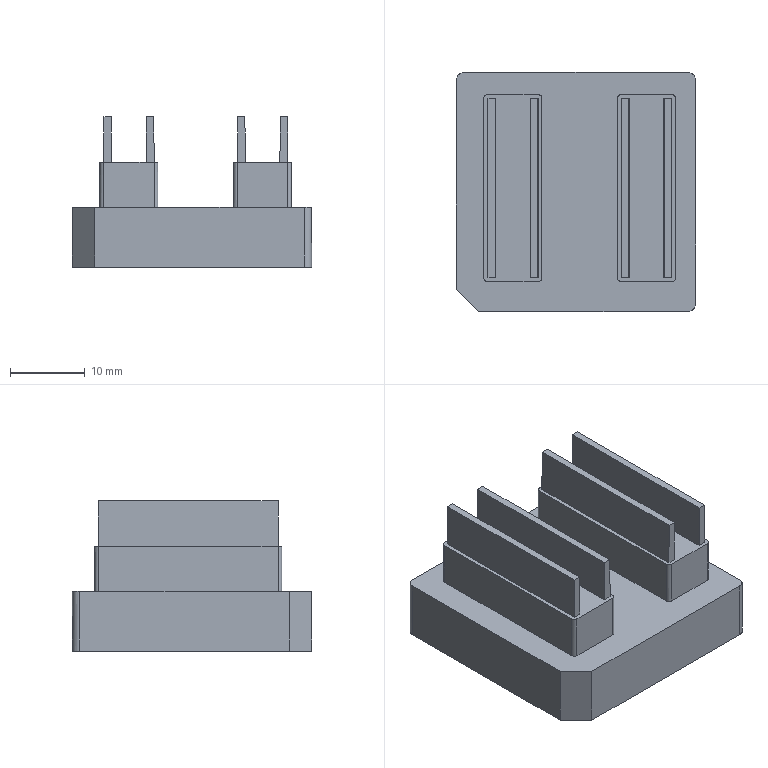NC program | PowerMill | posted with a generic post | part box 32 x 32 x 20.109 mm
Lines 5927 to 6909 of 124326:
N6024 M6
N6025 S18000 M03
N6026 G00 G90 X0.0 Y0.0
N6027 G43 Z9.7992 H10
N6028
N6029 G05 P10000 R4
N6030 X-8.0366 Y14.4474
N6031 Z0.8417
N6032 G01 Z-0.3583 F3000.0
N6033 X-8.0407 Y14.4286 F5000.0
N6034 G03 X-7.9079 Y14.2227 I0.1694 J-0.0366
N6035 G01 X-6.5639 Y13.9322
N6036 X-6.332 Y13.9917
N6037 X-5.0656 Y14.0127
N6038 X-4.6435 Y13.9367
N6039 X-4.2213 Y13.7119
N6040 X-3.9916 Y13.5083
N6041 X-3.7992 Y13.2347
N6042 X-3.7268 Y13.0861
N6043 X-3.6258 Y12.664
N6044 X-3.6132 Y12.2419
N6045 Y-11.3976
N6046 X-3.6515 Y-11.8197
N6047 X-3.7992 Y-12.2357
N6048 X-4.155 Y-12.664
N6049 X-4.6435 Y-12.9367
N6050 X-5.0656 Y-13.0127
N6051 X-6.332 Y-12.992
N6052 X-6.7541 Y-12.8517
N6053 X-7.0361 Y-12.664
N6054 X-7.1763 Y-12.536
N6055 X-7.3878 Y-12.2419
N6056 X-7.545 Y-11.8197
N6057 X-7.578 Y-11.3976
N6058 Y12.2419
N6059 X-7.5711 Y12.664
N6060 X-7.4587 Y13.0861
N6061 X-7.1989 Y13.5083
N6062 X-6.7541 Y13.8445
N6063 X-6.5711 Y13.9304
N6064 X-6.5639 Y13.9322
N6065 X-9.1258 Y14.4424
N6066 X-9.1676 Y14.2545
N6067 X-9.4274 Y13.0861
N6068 X-9.322 Y12.664
N6069 X-9.3158 Y12.2419
N6070 Y-11.3976
N6071 X-9.3507 Y-11.8197
N6072 X-9.5077 Y-12.2419
N6073 X-9.7091 Y-12.5237
N6074 X-9.8512 Y-12.664
N6075 X-10.1312 Y-12.8478
N6076 X-10.5533 Y-12.9903
N6077 X-10.9755 Y-13.0134
N6078 X-11.8197 Y-13.0124
N6079 X-12.2419 Y-12.9398
N6080 X-12.664 Y-12.7219
N6081 X-13.0861 Y-12.2457
N6082 X-13.2442 Y-11.8197
N6083 X-13.2724 Y-11.3976
N6084 X-13.2704 Y12.664
N6085 X-13.1589 Y13.0861
N6086 X-13.0861 Y13.2475
N6087 X-12.9007 Y13.5083
N6088 X-12.664 Y13.7232
N6089 X-12.2636 Y13.9304
N6090 X-11.8197 Y14.0127
N6091 X-10.9755 Y14.0134
N6092 X-10.5533 Y13.9902
N6093 X-10.3233 Y13.9304
N6094 X-10.1312 Y13.8488
N6095 X-9.7091 Y13.525
N6096 X-9.4274 Y13.0861
N6097 X-8.0426 Y14.447 Z-0.5056
N6098 X-8.0466 Y14.4282
N6099 G03 X-7.9139 Y14.2222 I0.1693 J-0.0367
N6100 G01 X-6.5688 Y13.9313
N6101 X-6.332 Y13.992
N6102 X-5.0656 Y14.0127
N6103 X-4.6435 Y13.9379
N6104 X-4.2213 Y13.7157
N6105 X-3.99 Y13.5083
N6106 X-3.7992 Y13.2376
N6107 X-3.7255 Y13.0861
N6108 X-3.6236 Y12.664
N6109 X-3.6119 Y12.2419
N6110 Y-11.3976
N6111 X-3.6467 Y-11.8197
N6112 X-3.7992 Y-12.2386
N6113 X-4.1495 Y-12.664
N6114 X-4.6435 Y-12.9375
N6115 X-5.0656 Y-13.0127
N6116 X-6.332 Y-12.9922
N6117 X-6.7541 Y-12.8531
N6118 X-7.0383 Y-12.664
N6119 X-7.1763 Y-12.5374
N6120 X-7.3908 Y-12.2419
N6121 X-7.5485 Y-11.8197
N6122 X-7.5795 Y-11.3976
N6123 Y12.2419
N6124 X-7.5724 Y12.664
N6125 X-7.4617 Y13.0861
N6126 X-7.2013 Y13.5083
N6127 X-6.7541 Y13.8486
N6128 X-6.5724 Y13.9304
N6129 X-6.5688 Y13.9313
N6130 X-9.1247 Y14.4437
N6131 X-9.1662 Y14.2557
N6132 X-9.4247 Y13.0861
N6133 X-9.3187 Y12.664
N6134 X-9.3111 Y12.2419
N6135 Y-11.3976
N6136 X-9.3471 Y-11.8197
N6137 X-9.5043 Y-12.2419
N6138 X-9.7091 Y-12.5265
N6139 X-9.8496 Y-12.664
N6140 X-10.1312 Y-12.8505
N6141 X-10.5533 Y-12.9912
N6142 X-10.9755 Y-13.0134
N6143 X-11.8197 Y-13.0128
N6144 X-12.2419 Y-12.9403
N6145 X-12.664 Y-12.7233
N6146 X-12.7378 Y-12.664
N6147 X-13.0861 Y-12.2492
N6148 X-13.2466 Y-11.8197
N6149 X-13.2748 Y-11.3976
N6150 X-13.2717 Y12.664
N6151 X-13.1613 Y13.0861
N6152 X-13.0861 Y13.2497
N6153 X-12.9019 Y13.5083
N6154 X-12.664 Y13.7243
N6155 X-12.2673 Y13.9304
N6156 X-11.8197 Y14.0128
N6157 X-10.9755 Y14.0134
N6158 X-10.5533 Y13.9908
N6159 X-10.3188 Y13.9304
N6160 X-10.1312 Y13.8502
N6161 X-9.7091 Y13.5273
N6162 X-9.4247 Y13.0861
N6163 X-8.0446 Y14.4474 Z-0.6529
N6164 X-8.0486 Y14.4286
N6165 G03 X-7.916 Y14.2226 I0.1693 J-0.0367
N6166 G01 X-6.57 Y13.9313
N6167 X-6.332 Y13.9922
N6168 X-5.0656 Y14.0128
N6169 X-4.6435 Y13.9389
N6170 X-4.2213 Y13.7196
N6171 X-3.9884 Y13.5083
N6172 X-3.7992 Y13.2405
N6173 X-3.7243 Y13.0861
N6174 X-3.6213 Y12.664
N6175 X-3.6107 Y12.2419
N6176 Y-11.3976
N6177 X-3.6422 Y-11.8197
N6178 X-3.7992 Y-12.2415
N6179 X-4.1482 Y-12.664
N6180 X-4.6435 Y-12.9384
N6181 X-5.0656 Y-13.0128
N6182 X-6.332 Y-12.9924
N6183 X-6.7541 Y-12.8541
N6184 X-7.0406 Y-12.664
N6185 X-7.1763 Y-12.5387
N6186 X-7.3926 Y-12.2419
N6187 X-7.5498 Y-11.8197
N6188 X-7.581 Y-11.3976
N6189 Y12.2419
N6190 X-7.5737 Y12.664
N6191 X-7.4646 Y13.0861
N6192 X-7.2036 Y13.5083
N6193 X-6.7541 Y13.8527
N6194 X-6.5737 Y13.9304
N6195 X-6.57 Y13.9313
N6196 X-9.1236 Y14.4426
N6197 X-9.1652 Y14.2546
N6198 X-9.4235 Y13.0861
N6199 X-9.3174 Y12.664
N6200 X-9.3099 Y12.2419
N6201 Y-11.3976
N6202 X-9.3434 Y-11.8197
N6203 X-9.5009 Y-12.2419
N6204 X-9.7091 Y-12.5293
N6205 X-9.8479 Y-12.664
N6206 X-10.1312 Y-12.8512
N6207 X-10.5533 Y-12.9914
N6208 X-10.561 Y-12.9915
N6209 X-10.9755 Y-13.0133
N6210 X-11.8066 Y-13.0128
N6211 X-11.8197 Y-13.013
N6212 X-12.2419 Y-12.9407
N6213 X-12.664 Y-12.7248
N6214 X-12.742 Y-12.664
N6215 X-13.0861 Y-12.252
N6216 X-13.249 Y-11.8197
N6217 X-13.2772 Y-11.3976
N6218 Y11.8197
N6219 X-13.273 Y12.664
N6220 X-13.1637 Y13.0861
N6221 X-13.0861 Y13.252
N6222 X-12.9032 Y13.5083
N6223 X-12.664 Y13.7254
N6224 X-12.271 Y13.9304
N6225 X-11.8197 Y14.0128
N6226 X-11.8125 Y14.0127
N6227 X-10.9755 Y14.0133
N6228 X-10.5698 Y13.9917
N6229 X-10.5533 Y13.9914
N6230 X-10.3175 Y13.9304
N6231 X-10.1312 Y13.8512
N6232 X-9.7091 Y13.5296
N6233 X-9.4235 Y13.0861
N6234 X-8.0471 Y14.4479 Z-0.8002
N6235 X-8.0512 Y14.4291
N6236 G03 X-7.9186 Y14.2231 I0.1693 J-0.0367
N6237 G01 X-6.5713 Y13.9313
N6238 X-6.332 Y13.9925
N6239 X-5.0656 Y14.0129
N6240 X-4.6435 Y13.9393
N6241 X-4.2213 Y13.7224
N6242 X-3.9868 Y13.5083
N6243 X-3.7992 Y13.2434
N6244 X-3.723 Y13.0861
N6245 X-3.6191 Y12.664
N6246 X-3.6094 Y12.2419
N6247 Y-11.3976
N6248 X-3.641 Y-11.8197
N6249 X-3.7981 Y-12.2419
N6250 X-4.1469 Y-12.664
N6251 X-4.6435 Y-12.9393
N6252 X-5.0656 Y-13.0129
N6253 X-6.332 Y-12.9926
N6254 X-6.7541 Y-12.8548
N6255 X-7.0429 Y-12.664
N6256 X-7.1763 Y-12.5401
N6257 X-7.3939 Y-12.2419
N6258 X-7.551 Y-11.8197
N6259 X-7.5824 Y-11.3976
N6260 Y12.2419
N6261 X-7.575 Y12.664
N6262 X-7.4676 Y13.0861
N6263 X-7.2053 Y13.5083
N6264 X-6.7541 Y13.8548
N6265 X-6.575 Y13.9304
N6266 X-6.5713 Y13.9313
N6267 X-9.1222 Y14.443
N6268 X-9.1638 Y14.255
N6269 X-9.4222 Y13.0861
N6270 X-9.3161 Y12.664
N6271 X-9.3086 Y12.2419
N6272 Y-11.3976
N6273 X-9.3402 Y-11.8197
N6274 X-9.4975 Y-12.2419
N6275 X-9.7091 Y-12.5321
N6276 X-9.8462 Y-12.664
N6277 X-10.1312 Y-12.8518
N6278 X-10.5533 Y-12.9916
N6279 X-10.5686 Y-12.9919
N6280 X-10.9755 Y-13.0133
N6281 X-11.8019 Y-13.0127
N6282 X-11.8197 Y-13.013
N6283 X-12.2419 Y-12.9412
N6284 X-12.664 Y-12.7262
N6285 X-12.7443 Y-12.664
N6286 X-13.0861 Y-12.2543
N6287 X-13.2502 Y-11.8197
N6288 X-13.2796 Y-11.3976
N6289 Y12.2419
N6290 X-13.2743 Y12.664
N6291 X-13.1661 Y13.0861
N6292 X-13.0861 Y13.2543
N6293 X-12.9045 Y13.5083
N6294 X-12.664 Y13.7264
N6295 X-12.2742 Y13.9304
N6296 X-11.8197 Y14.0129
N6297 X-11.8052 Y14.0127
N6298 X-10.9755 Y14.0133
N6299 X-10.5772 Y13.992
N6300 X-10.5745
N6301 X-10.5533 Y13.9916
N6302 X-10.3162 Y13.9304
N6303 X-10.1312 Y13.8518
N6304 X-9.7091 Y13.5319
N6305 X-9.4222 Y13.0861
N6306 X-8.0487 Y14.4482 Z-0.9475
N6307 X-8.0528 Y14.4294
N6308 G03 X-7.9202 Y14.2234 I0.1693 J-0.0367
N6309 G01 X-6.5726 Y13.9313
N6310 X-6.332 Y13.9928
N6311 X-5.0656 Y14.0129
N6312 X-4.6435 Y13.9397
N6313 X-4.2213 Y13.7233
N6314 X-3.9854 Y13.5083
N6315 X-3.7992 Y13.2462
N6316 X-3.7217 Y13.0861
N6317 X-3.6169 Y12.664
N6318 X-3.6081 Y12.2419
N6319 Y-11.3976
N6320 X-3.6397 Y-11.8197
N6321 X-3.7968 Y-12.2419
N6322 X-4.1456 Y-12.664
N6323 X-4.2213 Y-12.7233
N6324 X-4.6435 Y-12.9397
N6325 X-5.0656 Y-13.0129
N6326 X-6.332 Y-12.9928
N6327 X-6.7541 Y-12.8554
N6328 X-7.0451 Y-12.664
N6329 X-7.1763 Y-12.5415
N6330 X-7.3952 Y-12.2419
N6331 X-7.5523 Y-11.8197
N6332 X-7.5839 Y-11.3976
N6333 Y12.2419
N6334 X-7.5763 Y12.664
N6335 X-7.4703 Y13.0861
N6336 X-7.2066 Y13.5083
N6337 X-6.7541 Y13.8554
N6338 X-6.5762 Y13.9304
N6339 X-6.5726 Y13.9313
N6340 X-9.1209 Y14.4433
N6341 X-9.1624 Y14.2553
N6342 X-9.4209 Y13.0861
N6343 X-9.3149 Y12.664
N6344 X-9.3073 Y12.2419
N6345 Y-11.3976
N6346 X-9.3389 Y-11.8197
N6347 X-9.496 Y-12.2419
N6348 X-9.7091 Y-12.5349
N6349 X-9.8448 Y-12.664
N6350 X-10.1312 Y-12.8525
N6351 X-10.5533 Y-12.9918
N6352 X-10.5761 Y-12.9922
N6353 X-10.5787 Y-12.9924
N6354 X-10.9755 Y-13.0132
N6355 X-11.797 Y-13.0127
N6356 X-11.8197 Y-13.013
N6357 X-12.2419 Y-12.9416
N6358 X-12.664 Y-12.7276
N6359 X-12.7456 Y-12.664
N6360 X-13.0861 Y-12.2565
N6361 X-13.2515 Y-11.8197
N6362 X-13.2819 Y-11.3976
N6363 Y12.2419
N6364 X-13.2755 Y12.664
N6365 X-13.1685 Y13.0861
N6366 X-13.0861 Y13.2565
N6367 X-12.9058 Y13.5083
N6368 X-12.664 Y13.7275
N6369 X-12.2754 Y13.9304
N6370 X-11.8197 Y14.013
N6371 X-11.7978 Y14.0126
N6372 X-10.9755 Y14.0132
N6373 X-10.5845 Y13.9924
N6374 X-10.5533 Y13.9918
N6375 X-10.315 Y13.9304
N6376 X-10.1312 Y13.8525
N6377 X-9.7091 Y13.5342
N6378 X-9.4209 Y13.0861
N6379 X-8.0495 Y14.4487 Z-1.0949
N6380 X-8.0535 Y14.4299
N6381 G03 X-7.921 Y14.2238 I0.1693 J-0.0368
N6382 G01 X-6.5738 Y13.9313
N6383 X-6.332 Y13.9931
N6384 X-5.0656 Y14.0129
N6385 X-4.6435 Y13.9401
N6386 X-4.2213 Y13.7243
N6387 X-3.9841 Y13.5083
N6388 X-3.7992 Y13.2484
N6389 X-3.7204 Y13.0861
N6390 X-3.6147 Y12.664
N6391 X-3.6068 Y12.2419
N6392 Y-11.3976
N6393 X-3.6384 Y-11.8197
N6394 X-3.7955 Y-12.2419
N6395 X-4.1443 Y-12.664
N6396 X-4.2213 Y-12.7243
N6397 X-4.6435 Y-12.9401
N6398 X-5.0656 Y-13.0129
N6399 X-6.332 Y-12.9931
N6400 X-6.7541 Y-12.8561
N6401 X-7.0474 Y-12.664
N6402 X-7.1763 Y-12.5429
N6403 X-7.3965 Y-12.2419
N6404 X-7.5536 Y-11.8197
N6405 X-7.5852 Y-11.3976
N6406 Y12.2419
N6407 X-7.5776 Y12.664
N6408 X-7.4716 Y13.0861
N6409 X-7.2079 Y13.5083
N6410 X-6.7541 Y13.8561
N6411 X-6.5775 Y13.9304
N6412 X-6.5738 Y13.9313
N6413 X-9.1195 Y14.4436
N6414 X-9.1611 Y14.2556
N6415 X-9.4196 Y13.0861
N6416 X-9.3136 Y12.664
N6417 X-9.306 Y12.2419
N6418 Y-11.3976
N6419 X-9.3376 Y-11.8197
N6420 X-9.4947 Y-12.2419
N6421 X-9.7091 Y-12.5366
N6422 X-9.8435 Y-12.664
N6423 X-10.1312 Y-12.8531
N6424 X-10.5533 Y-12.9921
N6425 X-10.5835 Y-12.9926
N6426 X-10.5862 Y-12.9927
N6427 X-10.9755 Y-13.0132
N6428 X-11.7921 Y-13.0126
N6429 X-11.8197 Y-13.0131
N6430 X-12.2419 Y-12.942
N6431 X-12.664 Y-12.7285
N6432 X-12.7469 Y-12.664
N6433 X-13.0861 Y-12.2588
N6434 X-13.2528 Y-11.8197
N6435 X-13.2843 Y-11.3976
N6436 Y12.2419
N6437 X-13.2768 Y12.664
N6438 X-13.1708 Y13.0861
N6439 X-13.0861 Y13.2588
N6440 X-12.9071 Y13.5083
N6441 X-12.664 Y13.7285
N6442 X-12.2767 Y13.9304
N6443 X-11.8197 Y14.0131
N6444 X-11.7902 Y14.0126
N6445 X-10.9755 Y14.0132
N6446 X-10.5918 Y13.9927
N6447 X-10.5533 Y13.9921
N6448 X-10.3137 Y13.9304
N6449 X-10.1312 Y13.8531
N6450 X-9.7091 Y13.5365
N6451 X-9.4196 Y13.0861
N6452 X-8.05 Y14.4493 Z-1.2422
N6453 X-8.0541 Y14.4304
N6454 G03 X-7.9216 Y14.2243 I0.1693 J-0.0368
N6455 G01 X-6.5751 Y13.9313
N6456 X-6.332 Y13.9933
N6457 X-5.0656 Y14.013
N6458 X-4.6435 Y13.9406
N6459 X-4.2213 Y13.7252
N6460 X-3.9828 Y13.5083
N6461 X-3.7992 Y13.2507
N6462 X-3.7191 Y13.0861
N6463 X-3.6131 Y12.664
N6464 X-3.6055 Y12.2419
N6465 Y-11.3976
N6466 X-3.6371 Y-11.8197
N6467 X-3.7942 Y-12.2419
N6468 X-4.143 Y-12.664
N6469 X-4.2213 Y-12.7252
N6470 X-4.6435 Y-12.9406
N6471 X-5.0656 Y-13.013
N6472 X-6.332 Y-12.9933
N6473 X-6.7541 Y-12.8567
N6474 X-7.049 Y-12.664
N6475 X-7.1763 Y-12.5442
N6476 X-7.3978 Y-12.2419
N6477 X-7.5549 Y-11.8197
N6478 X-7.5865 Y-11.3976
N6479 Y12.2419
N6480 X-7.5789 Y12.664
N6481 X-7.4729 Y13.0861
N6482 X-7.2092 Y13.5083
N6483 X-6.7541 Y13.8567
N6484 X-6.5788 Y13.9304
N6485 X-6.5751 Y13.9313
N6486 X-9.1182 Y14.4439
N6487 X-9.1597 Y14.2559
N6488 X-9.4183 Y13.0861
N6489 X-9.3123 Y12.664
N6490 X-9.3047 Y12.2419
N6491 Y-11.3976
N6492 X-9.3363 Y-11.8197
N6493 X-9.4934 Y-12.2419
N6494 X-9.7091 Y-12.538
N6495 X-9.8422 Y-12.664
N6496 X-10.1312 Y-12.8538
N6497 X-10.5533 Y-12.9923
N6498 X-10.5908 Y-12.9929
N6499 X-10.5935 Y-12.993
N6500 X-10.9755 Y-13.0131
N6501 X-11.7871 Y-13.0126
N6502 X-11.8197 Y-13.0131
N6503 X-12.2419 Y-12.9424
N6504 X-12.664 Y-12.7295
N6505 X-12.7482 Y-12.664
N6506 X-13.0861 Y-12.261
N6507 X-13.2541 Y-11.8197
N6508 X-13.2857 Y-11.3976
N6509 Y12.2419
N6510 X-13.2781 Y12.664
N6511 X-13.1721 Y13.0861
N6512 X-13.0861 Y13.261
N6513 X-12.9084 Y13.5083
N6514 X-12.664 Y13.7295
N6515 X-12.278 Y13.9304
N6516 X-11.8197 Y14.0131
N6517 X-11.7845 Y14.0125
N6518 X-10.9755 Y14.0131
N6519 X-10.5989 Y13.993
N6520 X-10.5533 Y13.9923
N6521 X-10.3124 Y13.9304
N6522 X-10.1312 Y13.8538
N6523 X-9.7091 Y13.538
N6524 X-9.4183 Y13.0861
N6525 X-8.0504 Y14.4498 Z-1.3895
N6526 X-8.0546 Y14.431
N6527 G03 X-7.9222 Y14.2248 I0.1693 J-0.0369
N6528 G01 X-6.5764 Y13.9313
N6529 X-6.332 Y13.9935
N6530 X-5.0656 Y14.013
N6531 X-4.6435 Y13.941
N6532 X-4.2213 Y13.7261
N6533 X-3.9815 Y13.5083
N6534 X-3.7992 Y13.253
N6535 X-3.7178 Y13.0861
N6536 X-3.6118 Y12.664
N6537 X-3.6042 Y12.2419
N6538 Y-11.3976
N6539 X-3.6358 Y-11.8197
N6540 X-3.7394 Y-12.0945
N6541 X-3.7943 Y-12.2418
N6542 X-3.7969 Y-12.2474
N6543 X-3.7992 Y-12.253
N6544 X-4.1418 Y-12.664
N6545 X-4.2213 Y-12.7261
N6546 X-4.6435 Y-12.941
N6547 X-5.0656 Y-13.013
N6548 X-6.332 Y-12.9935
N6549 X-6.7541 Y-12.8574
N6550 X-7.0502 Y-12.664
N6551 X-7.1763 Y-12.5456
N6552 X-7.3991 Y-12.2419
N6553 X-7.5562 Y-11.8197
N6554 X-7.5878 Y-11.3976
N6555 Y12.2419
N6556 X-7.5802 Y12.664
N6557 X-7.4742 Y13.0861
N6558 X-7.2105 Y13.5083
N6559 X-6.7541 Y13.8574
N6560 X-6.5801 Y13.9304
N6561 X-6.5764 Y13.9313
N6562 X-9.1168 Y14.4442
N6563 X-9.1584 Y14.2562
N6564 X-9.417 Y13.0861
N6565 X-9.311 Y12.664
N6566 X-9.3034 Y12.2419
N6567 Y-11.3976
N6568 X-9.335 Y-11.8197
N6569 X-9.4921 Y-12.2419
N6570 X-9.7091 Y-12.5393
N6571 X-9.841 Y-12.664
N6572 X-10.1312 Y-12.8544
N6573 X-10.5533 Y-12.9925
N6574 X-10.598 Y-12.9932
N6575 X-10.9755 Y-13.0131
N6576 X-11.7823 Y-13.0125
N6577 X-11.8197 Y-13.0131
N6578 X-12.2419 Y-12.9429
N6579 X-12.664 Y-12.7304
N6580 X-12.7494 Y-12.664
N6581 X-13.0861 Y-12.2632
N6582 X-13.2554 Y-11.8197
N6583 X-13.287 Y-11.3976
N6584 Y12.2419
N6585 X-13.2794 Y12.664
N6586 X-13.1734 Y13.0861
N6587 X-13.0861 Y13.2633
N6588 X-12.9097 Y13.5083
N6589 X-12.664 Y13.7304
N6590 X-12.2793 Y13.9304
N6591 X-11.8197 Y14.0131
N6592 X-11.7797 Y14.0125
N6593 X-10.9755 Y14.0131
N6594 X-10.606 Y13.9934
N6595 X-10.6032 Y13.9933
N6596 X-10.5533 Y13.9925
N6597 X-10.3111 Y13.9304
N6598 X-10.1312 Y13.8544
N6599 X-9.7091 Y13.5393
N6600 X-9.417 Y13.0861
N6601 X-8.0509 Y14.4503 Z-1.5368
N6602 X-8.055 Y14.4315
N6603 G03 X-7.9227 Y14.2252 I0.1692 J-0.037
N6604 G01 X-6.5776 Y13.9313
N6605 X-6.332 Y13.9937
N6606 X-5.0656 Y14.013
N6607 X-4.6435 Y13.9414
N6608 X-4.2213 Y13.7271
N6609 X-3.9803 Y13.5083
N6610 X-3.7992 Y13.2553
N6611 X-3.7165 Y13.0861
N6612 X-3.6105 Y12.664
N6613 X-3.6029 Y12.2419
N6614 Y-11.3976
N6615 X-3.6345 Y-11.8197
N6616 X-3.7917 Y-12.2419
N6617 X-3.7956 Y-12.2473
N6618 X-3.7992 Y-12.253
N6619 X-3.9851 Y-12.4759
N6620 X-4.1405 Y-12.664
N6621 X-4.2213 Y-12.7271
N6622 X-4.6435 Y-12.9414
N6623 X-5.0656 Y-13.013
N6624 X-6.332 Y-12.9937
N6625 X-6.7541 Y-12.858
N6626 X-7.0515 Y-12.664
N6627 X-7.1763 Y-12.5469
N6628 X-7.4003 Y-12.2419
N6629 X-7.5575 Y-11.8197
N6630 X-7.5891 Y-11.3976
N6631 Y12.2419
N6632 X-7.5815 Y12.664
N6633 X-7.4755 Y13.0861
N6634 X-7.2117 Y13.5083
N6635 X-6.7541 Y13.858
N6636 X-6.5814 Y13.9304
N6637 X-6.5776 Y13.9313
N6638 X-9.1155 Y14.4445
N6639 X-9.157 Y14.2565
N6640 X-9.4157 Y13.0861
N6641 X-9.3097 Y12.664
N6642 X-9.3021 Y12.2419
N6643 Y-11.3976
N6644 X-9.3337 Y-11.8197
N6645 X-9.4909 Y-12.2419
N6646 X-9.7091 Y-12.5407
N6647 X-9.8397 Y-12.664
N6648 X-10.1312 Y-12.8551
N6649 X-10.5533 Y-12.9927
N6650 X-10.6052 Y-12.9936
N6651 X-10.9755 Y-13.013
N6652 X-11.7774 Y-13.0125
N6653 X-11.7787
N6654 X-11.8197 Y-13.0132
N6655 X-12.2419 Y-12.9433
N6656 X-12.664 Y-12.7313
N6657 X-12.7507 Y-12.664
N6658 X-13.0861 Y-12.2655
N6659 X-13.2567 Y-11.8197
N6660 X-13.2883 Y-11.3976
N6661 Y12.2419
N6662 X-13.2807 Y12.664
N6663 X-13.1747 Y13.0861
N6664 X-13.0861 Y13.2655
N6665 X-12.9109 Y13.5083
N6666 X-12.664 Y13.7313
N6667 X-12.2806 Y13.9304
N6668 X-11.8197 Y14.0132
N6669 X-11.7748 Y14.0124
N6670 X-10.9755 Y14.013
N6671 X-10.6129 Y13.9937
N6672 X-10.5533 Y13.9927
N6673 X-10.3098 Y13.9304
N6674 X-10.1312 Y13.8551
N6675 X-9.7091 Y13.5407
N6676 X-9.4157 Y13.0861
N6677 X-8.0523 Y14.451 Z-1.6841
N6678 X-8.0564 Y14.4322
N6679 G03 X-7.9242 Y14.2259 I0.1693 J-0.0371
N6680 G01 X-6.5789 Y13.9314
N6681 X-6.332 Y13.9939
N6682 X-5.0656 Y14.0131
N6683 X-4.6435 Y13.9418
N6684 X-4.2213 Y13.728
N6685 X-3.979 Y13.5083
N6686 X-3.7992 Y13.2575
N6687 X-3.7153 Y13.0861
N6688 X-3.6092 Y12.664
N6689 X-3.6017 Y12.2419
N6690 Y-11.3976
N6691 X-3.6332 Y-11.8197
N6692 X-3.7904 Y-12.2419
N6693 X-3.7991 Y-12.2524
N6694 X-3.7993 Y-12.253
N6695 X-3.8284 Y-12.2879
N6696 X-4.1392 Y-12.664
N6697 X-4.2213 Y-12.728
N6698 X-4.6435 Y-12.9418
N6699 X-5.0656 Y-13.0131
N6700 X-6.332 Y-12.9939
N6701 X-6.7541 Y-12.8586
N6702 X-7.0528 Y-12.664
N6703 X-7.1763 Y-12.5483
N6704 X-7.4016 Y-12.2419
N6705 X-7.5588 Y-11.8197
N6706 X-7.5903 Y-11.3976
N6707 Y12.2419
N6708 X-7.5828 Y12.664
N6709 X-7.4767 Y13.0861
N6710 X-7.213 Y13.5083
N6711 X-6.7541 Y13.8586
N6712 X-6.5827 Y13.9304
N6713 X-6.5789 Y13.9314
N6714 X-9.1141 Y14.4449
N6715 X-9.1557 Y14.2569
N6716 X-9.4145 Y13.0861
N6717 X-9.3084 Y12.664
N6718 X-9.3009 Y12.2419
N6719 Y-11.3976
N6720 X-9.3324 Y-11.8197
N6721 X-9.4896 Y-12.2419
N6722 X-9.7091 Y-12.5421
N6723 X-9.8384 Y-12.664
N6724 X-10.1312 Y-12.8557
N6725 X-10.5533 Y-12.9929
N6726 X-10.6122 Y-12.9939
N6727 X-10.9755 Y-13.013
N6728 X-11.7724 Y-13.0124
N6729 X-11.7736 Y-13.0125
N6730 X-11.8197 Y-13.0132
N6731 X-12.2419 Y-12.9437
N6732 X-12.664 Y-12.7322
N6733 X-12.752 Y-12.664
N6734 X-13.0861 Y-12.2677
N6735 X-13.258 Y-11.8197
N6736 X-13.2895 Y-11.3976
N6737 Y12.2419
N6738 X-13.282 Y12.664
N6739 X-13.1759 Y13.0861
N6740 X-13.0861 Y13.2677
N6741 X-12.9122 Y13.5083
N6742 X-12.664 Y13.7322
N6743 X-12.2819 Y13.9304
N6744 X-11.8197 Y14.0132
N6745 X-11.7698 Y14.0124
N6746 X-10.9755 Y14.013
N6747 X-10.6198 Y13.994
N6748 X-10.5533 Y13.9929
N6749 X-10.3085 Y13.9304
N6750 X-10.1312 Y13.8557
N6751 X-9.7091 Y13.5421
N6752 X-9.4145 Y13.0861
N6753 X-8.0527 Y14.4515 Z-1.8314
N6754 X-8.0568 Y14.4327
N6755 G03 X-7.9247 Y14.2264 I0.1692 J-0.0371
N6756 G01 X-6.5802 Y13.9314
N6757 X-6.332 Y13.9941
N6758 X-5.0656 Y14.0131
N6759 X-4.6435 Y13.9422
N6760 X-4.2213 Y13.7289
N6761 X-3.9777 Y13.5083
N6762 X-3.7992 Y13.2598
N6763 X-3.714 Y13.0861
N6764 X-3.6079 Y12.664
N6765 X-3.6004 Y12.2419
N6766 Y-11.3976
N6767 X-3.632 Y-11.8197
N6768 X-3.7891 Y-12.2419
N6769 X-4.1379 Y-12.664
N6770 X-4.2213 Y-12.7289
N6771 X-4.6435 Y-12.9422
N6772 X-5.0656 Y-13.0131
N6773 X-6.332 Y-12.9941
N6774 X-6.7541 Y-12.8593
N6775 X-7.0541 Y-12.664
N6776 X-7.1763 Y-12.5496
N6777 X-7.4029 Y-12.2419
N6778 X-7.56 Y-11.8197
N6779 X-7.5916 Y-11.3976
N6780 Y12.2419
N6781 X-7.5841 Y12.664
N6782 X-7.478 Y13.0861
N6783 X-7.2143 Y13.5083
N6784 X-6.7541 Y13.8593
N6785 X-6.584 Y13.9304
N6786 X-6.5802 Y13.9314
N6787 X-9.1128 Y14.4452
N6788 X-9.1543 Y14.2572
N6789 X-9.4132 Y13.0861
N6790 X-9.3071 Y12.664
N6791 X-9.2996 Y12.2419
N6792 Y-11.3976
N6793 X-9.3312 Y-11.8197
N6794 X-9.4883 Y-12.2419
N6795 X-9.7091 Y-12.5434
N6796 X-9.8371 Y-12.664
N6797 X-10.1312 Y-12.8564
N6798 X-10.5533 Y-12.9931
N6799 X-10.6191 Y-12.9942
N6800 X-10.9755 Y-13.0129
N6801 X-11.7674 Y-13.0124
N6802 X-11.7686
N6803 X-11.8197 Y-13.0132
N6804 X-12.2419 Y-12.9441
N6805 X-12.664 Y-12.7332
N6806 X-12.7533 Y-12.664
N6807 X-13.0861 Y-12.2699
N6808 X-13.2592 Y-11.8197
N6809 X-13.2908 Y-11.3976
N6810 Y12.2419
N6811 X-13.2833 Y12.664
N6812 X-13.1772 Y13.0861
N6813 X-13.0861 Y13.2699
N6814 X-12.9135 Y13.5083
N6815 X-12.664 Y13.7332
N6816 X-12.2832 Y13.9304
N6817 X-11.8197 Y14.0132
N6818 X-11.7647 Y14.0123
N6819 X-10.9755 Y14.0129
N6820 X-10.6266 Y13.9943
N6821 X-10.5533 Y13.9931
N6822 X-10.3072 Y13.9304
N6823 X-10.1312 Y13.8564
N6824 X-9.7091 Y13.5434
N6825 X-9.4132 Y13.0861
N6826 X-8.0533 Y14.452 Z-1.9787
N6827 X-8.0574 Y14.4332
N6828 G03 X-7.9254 Y14.2268 I0.1692 J-0.0372
N6829 G01 X-6.5814 Y13.9314
N6830 X-6.332 Y13.9943
N6831 X-5.0656 Y14.0131
N6832 X-4.6435 Y13.9426
N6833 X-4.2213 Y13.7299
N6834 X-3.9764 Y13.5083
N6835 X-3.7992 Y13.262
N6836 X-3.7127 Y13.0861
N6837 X-3.6067 Y12.664
N6838 X-3.5991 Y12.2419
N6839 Y-11.3976
N6840 X-3.6307 Y-11.8197
N6841 X-3.7878 Y-12.2419
N6842 X-4.1366 Y-12.664
N6843 X-4.2213 Y-12.7299
N6844 X-4.6435 Y-12.9426
N6845 X-5.0656 Y-13.0131
N6846 X-6.332 Y-12.9943
N6847 X-6.7541 Y-12.8599
N6848 X-7.0554 Y-12.664
N6849 X-7.1763 Y-12.551
N6850 X-7.4042 Y-12.2419
N6851 X-7.5613 Y-11.8197
N6852 X-7.5929 Y-11.3976
N6853 Y12.2419
N6854 X-7.5853 Y12.664
N6855 X-7.4793 Y13.0861
N6856 X-7.2156 Y13.5083
N6857 X-6.7541 Y13.8599
N6858 X-6.5852 Y13.9304
N6859 X-6.5814 Y13.9314
N6860 X-9.1114 Y14.4455
N6861 X-9.153 Y14.2575
N6862 X-9.4119 Y13.0861
N6863 X-9.3059 Y12.664
N6864 X-9.2983 Y12.2419
N6865 Y-11.3976
N6866 X-9.3299 Y-11.8197
N6867 X-9.487 Y-12.2419
N6868 X-9.7091 Y-12.5448
N6869 X-9.8358 Y-12.664
N6870 X-10.1312 Y-12.857
N6871 X-10.5533 Y-12.9934
N6872 X-10.626 Y-12.9945
N6873 X-10.9755 Y-13.0129
N6874 X-11.7623 Y-13.0123
N6875 X-11.7635 Y-13.0124
N6876 X-11.8197 Y-13.0132
N6877 X-12.2419 Y-12.9445
N6878 X-12.664 Y-12.7341
N6879 X-12.7546 Y-12.664
N6880 X-13.0861 Y-12.2721
N6881 X-13.2605 Y-11.8197
N6882 X-13.2921 Y-11.3976
N6883 Y12.2419
N6884 X-13.2845 Y12.664
N6885 X-13.1785 Y13.0861
N6886 X-13.0861 Y13.2721
N6887 X-12.9148 Y13.5083
N6888 X-12.664 Y13.7341
N6889 X-12.2844 Y13.9304
N6890 X-11.8197 Y14.0132
N6891 X-11.7597 Y14.0123
N6892 X-10.9755 Y14.0129
N6893 X-10.6332 Y13.9946
N6894 X-10.5533 Y13.9934
N6895 X-10.306 Y13.9304
N6896 X-10.1312 Y13.857
N6897 X-9.7091 Y13.5448
N6898 X-9.4119 Y13.0861
N6899 X-8.0537 Y14.4526 Z-2.126
N6900 X-8.0578 Y14.4338
N6901 G03 X-7.9259 Y14.2273 I0.1692 J-0.0373
N6902 G01 X-6.5827 Y13.9314
N6903 X-6.332 Y13.9945
N6904 X-5.0656 Y14.0131
N6905 X-4.6435 Y13.943
N6906 X-4.2213 Y13.7308
N6907 X-3.9751 Y13.5083
N6908 X-3.7992 Y13.2642
N6909 X-3.7114 Y13.0861
N6910 X-3.6054 Y12.664
N6911 X-3.5978 Y12.2419
N6912 Y-11.3976
N6913 X-3.6294 Y-11.8197
N6914 X-3.7865 Y-12.2419
N6915 X-4.1353 Y-12.664
N6916 X-4.2213 Y-12.7308
N6917 X-4.6435 Y-12.943
N6918 X-5.0656 Y-13.0131
N6919 X-6.332 Y-12.9945
N6920 X-6.7541 Y-12.8605
N6921 X-7.0567 Y-12.664
N6922 X-7.1763 Y-12.5523
N6923 X-7.4055 Y-12.2419
N6924 X-7.5626 Y-11.8197
N6925 X-7.5942 Y-11.3976
N6926 Y12.2419
N6927 X-7.5866 Y12.664
N6928 X-7.4806 Y13.0861
N6929 X-7.2169 Y13.5083
N6930 X-6.7541 Y13.8605
N6931 X-6.5865 Y13.9304
N6932 X-6.5827 Y13.9314
N6933 X-9.1101 Y14.4458
N6934 X-9.1516 Y14.2578
N6935 X-9.4106 Y13.0861
N6936 X-9.3046 Y12.664
N6937 X-9.297 Y12.2419
N6938 Y-11.3976
N6939 X-9.3286 Y-11.8197
N6940 X-9.4857 Y-12.2419
N6941 X-9.7091 Y-12.5462
N6942 X-9.8345 Y-12.664
N6943 X-10.1312 Y-12.8576
N6944 X-10.5533 Y-12.9936
N6945 X-10.6327 Y-12.9948
N6946 X-10.9755 Y-13.0128
N6947 X-11.7574 Y-13.0123
N6948 X-11.7586
N6949 X-11.8197 Y-13.0133
N6950 X-12.2419 Y-12.9449
N6951 X-12.664 Y-12.735
N6952 X-12.7559 Y-12.664
N6953 X-13.0861 Y-12.2743
N6954 X-13.2618 Y-11.8197
N6955 X-13.2934 Y-11.3976
N6956 Y12.2419
N6957 X-13.2858 Y12.664
N6958 X-13.1798 Y13.0861
N6959 X-13.0861 Y13.2743
N6960 X-12.9161 Y13.5083
N6961 X-12.664 Y13.735
N6962 X-12.2857 Y13.9304
N6963 X-11.8197 Y14.0133
N6964 X-11.7548 Y14.0123
N6965 X-10.9755 Y14.0128
N6966 X-10.6399 Y13.9949
N6967 X-10.5533 Y13.9936
N6968 X-10.3047 Y13.9304
N6969 X-10.1312 Y13.8576
N6970 X-9.7091 Y13.5462
N6971 X-9.4106 Y13.0861
N6972 X-8.0541 Y14.4531 Z-2.2734
N6973 X-8.0583 Y14.4343
N6974 G03 X-7.9265 Y14.2277 I0.1692 J-0.0374
N6975 G01 X-6.584 Y13.9314
N6976 X-6.332 Y13.9947
N6977 X-5.0656 Y14.0132
N6978 X-4.6435 Y13.9434
N6979 X-4.2213 Y13.7317
N6980 X-3.9738 Y13.5083
N6981 X-3.7992 Y13.2664
N6982 X-3.7101 Y13.0861
N6983 X-3.6041 Y12.664
N6984 X-3.5965 Y12.2419
N6985 Y-11.3976
N6986 X-3.6281 Y-11.8197
N6987 X-3.7852 Y-12.2419
N6988 X-4.134 Y-12.664
N6989 X-4.2213 Y-12.7317
N6990 X-4.6435 Y-12.9434
N6991 X-5.0656 Y-13.0132
N6992 X-6.332 Y-12.9947
N6993 X-6.7541 Y-12.8612
N6994 X-7.058 Y-12.664
N6995 X-7.1763 Y-12.5536
N6996 X-7.4068 Y-12.2419
N6997 X-7.5639 Y-11.8197
N6998 X-7.5955 Y-11.3976
N6999 Y12.2419
N7000 X-7.5879 Y12.664
N7001 X-7.4819 Y13.0861
N7002 X-7.2182 Y13.5083
N7003 X-6.7541 Y13.8611
N7004 X-6.5878 Y13.9304
N7005 X-6.584 Y13.9314
N7006 X-9.1087 Y14.4461